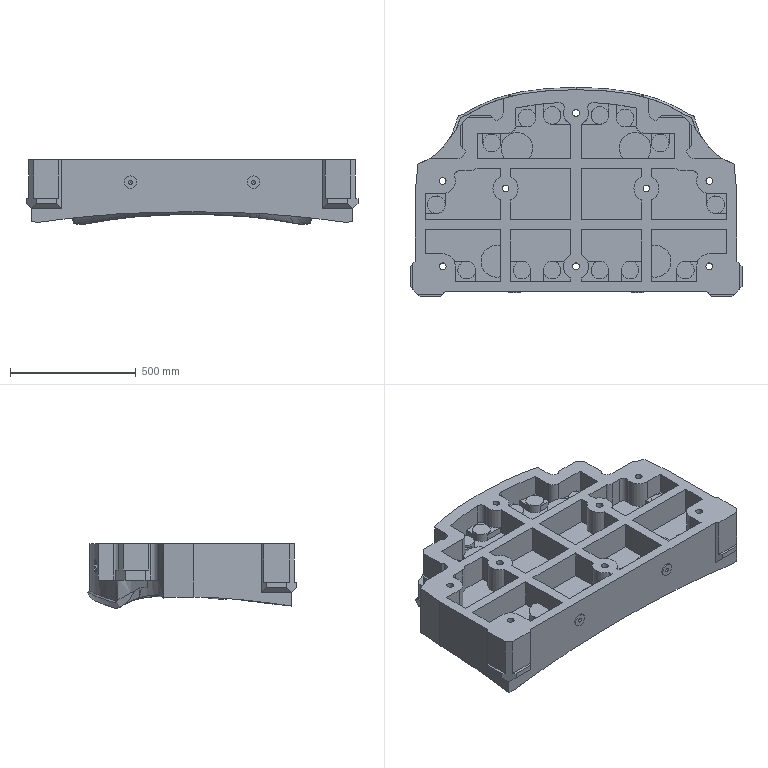Part | NX | features solid 2 | 3 solids | 460 faces | box 1320 x 831.905 x 257.83 mm | volume 103011649 mm3 | plane 226 | spline 142 | cylinder 88 | cone 4 | commonest cylinder face diameters 60 x20 100 x16 70 x14 40 x12 27 x8 50 x6